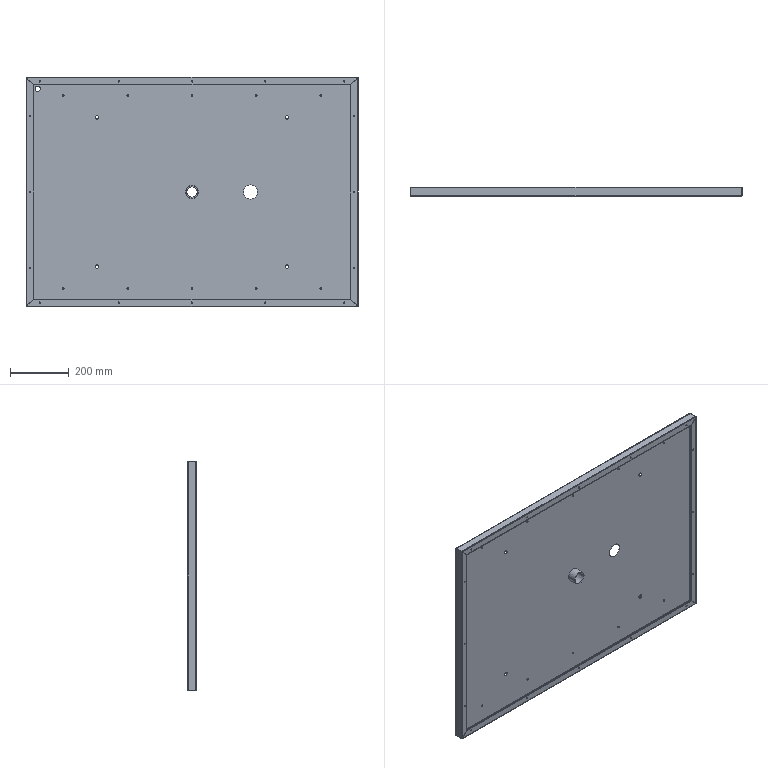Part | SolidWorks | features ICE 4, EdgeFlange 2, HoleWzd 2, Cut 1, FlatPattern 1, SMBaseFlange 1, SheetMetal 1, WeldmentFeature 1 | 2 solids | 142 faces | box 1135 x 31.2 x 785 mm | volume 1303037 mm3 | cylinder 86 | plane 40 | spline 16 | commonest cylinder face diameters 4 x32 5 x20 2 x8 4.4 x8 12 x8 18 x2